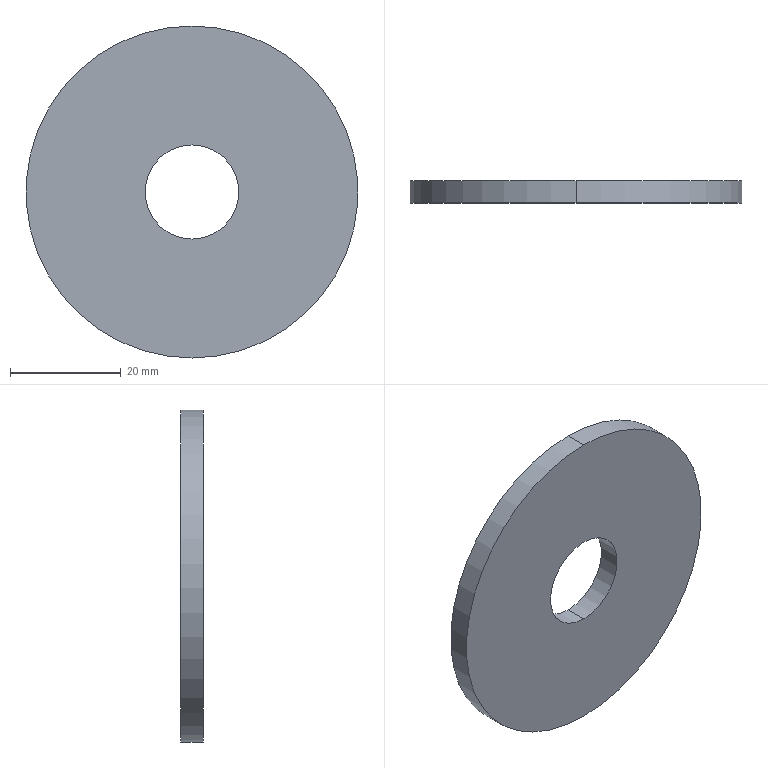Part | SolidWorks | features Extrusion 1 | 1 solid | 6 faces | box 60 x 4 x 60 mm | volume 10402 mm3 | cylinder 4 | plane 2 | commonest cylinder face diameters 17 x2 60 x2
STEP:
#1=CARTESIAN_POINT('',(0.,2.,-8.5));
#2=VERTEX_POINT('',#1);
#3=CARTESIAN_POINT('',(0.,2.,8.5));
#4=VERTEX_POINT('',#3);
#5=CARTESIAN_POINT('',(0.,2.,0.));
#6=DIRECTION('',(0.,1.,0.));
#7=DIRECTION('',(0.,0.,1.));
#8=AXIS2_PLACEMENT_3D('',#5,#6,#7);
#9=CIRCLE('',#8,8.5);
#10=EDGE_CURVE('',#2,#4,#9,.T.);
#11=ORIENTED_EDGE('',*,*,#10,.T.);
#12=CARTESIAN_POINT('',(0.,-2.,8.5));
#13=VERTEX_POINT('',#12);
#14=CARTESIAN_POINT('',(0.,2.,8.5));
#15=DIRECTION('',(0.,-1.,0.));
#16=VECTOR('',#15,1000.);
#17=LINE('',#14,#16);
#18=EDGE_CURVE('',#4,#13,#17,.T.);
#19=ORIENTED_EDGE('',*,*,#18,.T.);
#20=CARTESIAN_POINT('',(0.,-2.,-8.5));
#21=VERTEX_POINT('',#20);
#22=CARTESIAN_POINT('',(0.,-2.,0.));
#23=DIRECTION('',(0.,1.,0.));
#24=DIRECTION('',(0.,0.,1.));
#25=AXIS2_PLACEMENT_3D('',#22,#23,#24);
#26=CIRCLE('',#25,8.5);
#27=EDGE_CURVE('',#21,#13,#26,.T.);
#28=ORIENTED_EDGE('',*,*,#27,.F.);
#29=CARTESIAN_POINT('',(0.,2.,-8.5));
#30=DIRECTION('',(0.,-1.,0.));
#31=VECTOR('',#30,1000.);
#32=LINE('',#29,#31);
#33=EDGE_CURVE('',#2,#21,#32,.T.);
#34=ORIENTED_EDGE('',*,*,#33,.F.);
#35=EDGE_LOOP('',(#11,#19,#28,#34));
#36=FACE_OUTER_BOUND('',#35,.T.);
#37=CARTESIAN_POINT('',(0.,2.,0.));
#38=DIRECTION('',(0.,-1.,0.));
#39=DIRECTION('',(0.,0.,-1.));
#40=AXIS2_PLACEMENT_3D('',#37,#38,#39);
#41=CYLINDRICAL_SURFACE('',#40,8.5);
#42=ADVANCED_FACE('',(#36),#41,.F.);
#43=CARTESIAN_POINT('',(0.,2.,30.));
#44=VERTEX_POINT('',#43);
#45=CARTESIAN_POINT('',(0.,2.,-30.));
#46=VERTEX_POINT('',#45);
#47=CARTESIAN_POINT('',(0.,2.,0.));
#48=DIRECTION('',(0.,1.,0.));
#49=DIRECTION('',(0.,0.,1.));
#50=AXIS2_PLACEMENT_3D('',#47,#48,#49);
#51=CIRCLE('',#50,30.);
#52=EDGE_CURVE('',#44,#46,#51,.T.);
#53=ORIENTED_EDGE('',*,*,#52,.F.);
#54=CARTESIAN_POINT('',(0.,-2.,30.));
#55=VERTEX_POINT('',#54);
#56=CARTESIAN_POINT('',(0.,2.,30.));
#57=DIRECTION('',(0.,-1.,0.));
#58=VECTOR('',#57,1000.);
#59=LINE('',#56,#58);
#60=EDGE_CURVE('',#44,#55,#59,.T.);
#61=ORIENTED_EDGE('',*,*,#60,.T.);
#62=CARTESIAN_POINT('',(0.,-2.,-30.));
#63=VERTEX_POINT('',#62);
#64=CARTESIAN_POINT('',(0.,-2.,0.));
#65=DIRECTION('',(0.,1.,0.));
#66=DIRECTION('',(0.,0.,1.));
#67=AXIS2_PLACEMENT_3D('',#64,#65,#66);
#68=CIRCLE('',#67,30.);
#69=EDGE_CURVE('',#55,#63,#68,.T.);
#70=ORIENTED_EDGE('',*,*,#69,.T.);
#71=CARTESIAN_POINT('',(0.,2.,-30.));
#72=DIRECTION('',(0.,-1.,0.));
#73=VECTOR('',#72,1000.);
#74=LINE('',#71,#73);
#75=EDGE_CURVE('',#46,#63,#74,.T.);
#76=ORIENTED_EDGE('',*,*,#75,.F.);
#77=EDGE_LOOP('',(#53,#61,#70,#76));
#78=FACE_OUTER_BOUND('',#77,.T.);
#79=CARTESIAN_POINT('',(0.,2.,0.));
#80=DIRECTION('',(0.,-1.,0.));
#81=DIRECTION('',(0.,0.,-1.));
#82=AXIS2_PLACEMENT_3D('',#79,#80,#81);
#83=CYLINDRICAL_SURFACE('',#82,30.);
#84=ADVANCED_FACE('',(#78),#83,.T.);
#85=CARTESIAN_POINT('',(0.,2.,0.));
#86=DIRECTION('',(0.,1.,0.));
#87=DIRECTION('',(0.,0.,1.));
#88=AXIS2_PLACEMENT_3D('',#85,#86,#87);
#89=CIRCLE('',#88,30.);
#90=EDGE_CURVE('',#46,#44,#89,.T.);
#91=ORIENTED_EDGE('',*,*,#90,.T.);
#92=ORIENTED_EDGE('',*,*,#52,.T.);
#93=EDGE_LOOP('',(#91,#92));
#94=FACE_OUTER_BOUND('',#93,.T.);
#95=ORIENTED_EDGE('',*,*,#10,.F.);
#96=CARTESIAN_POINT('',(0.,2.,0.));
#97=DIRECTION('',(0.,1.,0.));
#98=DIRECTION('',(0.,0.,1.));
#99=AXIS2_PLACEMENT_3D('',#96,#97,#98);
#100=CIRCLE('',#99,8.5);
#101=EDGE_CURVE('',#4,#2,#100,.T.);
#102=ORIENTED_EDGE('',*,*,#101,.F.);
#103=EDGE_LOOP('',(#95,#102));
#104=FACE_BOUND('',#103,.T.);
#105=CARTESIAN_POINT('',(0.,2.,0.));
#106=DIRECTION('',(0.,1.,0.));
#107=DIRECTION('',(0.,0.,1.));
#108=AXIS2_PLACEMENT_3D('',#105,#106,#107);
#109=PLANE('',#108);
#110=ADVANCED_FACE('',(#94,#104),#109,.T.);
#111=CARTESIAN_POINT('',(0.,-2.,0.));
#112=DIRECTION('',(0.,1.,0.));
#113=DIRECTION('',(0.,0.,1.));
#114=AXIS2_PLACEMENT_3D('',#111,#112,#113);
#115=CIRCLE('',#114,30.);
#116=EDGE_CURVE('',#63,#55,#115,.T.);
#117=ORIENTED_EDGE('',*,*,#116,.F.);
#118=ORIENTED_EDGE('',*,*,#69,.F.);
#119=EDGE_LOOP('',(#117,#118));
#120=FACE_OUTER_BOUND('',#119,.T.);
#121=ORIENTED_EDGE('',*,*,#27,.T.);
#122=CARTESIAN_POINT('',(0.,-2.,0.));
#123=DIRECTION('',(0.,1.,0.));
#124=DIRECTION('',(0.,0.,1.));
#125=AXIS2_PLACEMENT_3D('',#122,#123,#124);
#126=CIRCLE('',#125,8.5);
#127=EDGE_CURVE('',#13,#21,#126,.T.);
#128=ORIENTED_EDGE('',*,*,#127,.T.);
#129=EDGE_LOOP('',(#121,#128));
#130=FACE_BOUND('',#129,.T.);
#131=CARTESIAN_POINT('',(0.,-2.,0.));
#132=DIRECTION('',(0.,1.,0.));
#133=DIRECTION('',(0.,0.,1.));
#134=AXIS2_PLACEMENT_3D('',#131,#132,#133);
#135=PLANE('',#134);
#136=ADVANCED_FACE('',(#120,#130),#135,.F.);
#137=ORIENTED_EDGE('',*,*,#60,.F.);
#138=ORIENTED_EDGE('',*,*,#90,.F.);
#139=ORIENTED_EDGE('',*,*,#75,.T.);
#140=ORIENTED_EDGE('',*,*,#116,.T.);
#141=EDGE_LOOP('',(#137,#138,#139,#140));
#142=FACE_OUTER_BOUND('',#141,.T.);
#143=CARTESIAN_POINT('',(0.,2.,0.));
#144=DIRECTION('',(0.,-1.,0.));
#145=DIRECTION('',(0.,0.,-1.));
#146=AXIS2_PLACEMENT_3D('',#143,#144,#145);
#147=CYLINDRICAL_SURFACE('',#146,30.);
#148=ADVANCED_FACE('',(#142),#147,.T.);
#149=ORIENTED_EDGE('',*,*,#18,.F.);
#150=ORIENTED_EDGE('',*,*,#101,.T.);
#151=ORIENTED_EDGE('',*,*,#33,.T.);
#152=ORIENTED_EDGE('',*,*,#127,.F.);
#153=EDGE_LOOP('',(#149,#150,#151,#152));
#154=FACE_OUTER_BOUND('',#153,.T.);
#155=CARTESIAN_POINT('',(0.,2.,0.));
#156=DIRECTION('',(0.,-1.,0.));
#157=DIRECTION('',(0.,0.,-1.));
#158=AXIS2_PLACEMENT_3D('',#155,#156,#157);
#159=CYLINDRICAL_SURFACE('',#158,8.5);
#160=ADVANCED_FACE('',(#154),#159,.F.);
#161=CLOSED_SHELL('',(#42,#84,#110,#136,#148,#160));
#162=MANIFOLD_SOLID_BREP('',#161);
#163=CARTESIAN_POINT('',(0.,0.,0.));
#164=DIRECTION('',(0.,0.,1.));
#165=DIRECTION('',(1.,0.,0.));
#166=AXIS2_PLACEMENT_3D('',#163,#164,#165);
#167=(LENGTH_UNIT()NAMED_UNIT(*)SI_UNIT(.MILLI.,.METRE.));
#168=UNCERTAINTY_MEASURE_WITH_UNIT(LENGTH_MEASURE(0.00001),#167,'','');
#169=(NAMED_UNIT(*)PLANE_ANGLE_UNIT()SI_UNIT($,.RADIAN.));
#170=(NAMED_UNIT(*)SI_UNIT($,.STERADIAN.)SOLID_ANGLE_UNIT());
#171=(GEOMETRIC_REPRESENTATION_CONTEXT(3)GLOBAL_UNCERTAINTY_ASSIGNED_CONTEXT((#168))GLOBAL_UNIT_ASSIGNED_CONTEXT((#167,#169,#170))REPRESENTATION_CONTEXT('',''));
#172=ADVANCED_BREP_SHAPE_REPRESENTATION('',(#162,#166),#171);